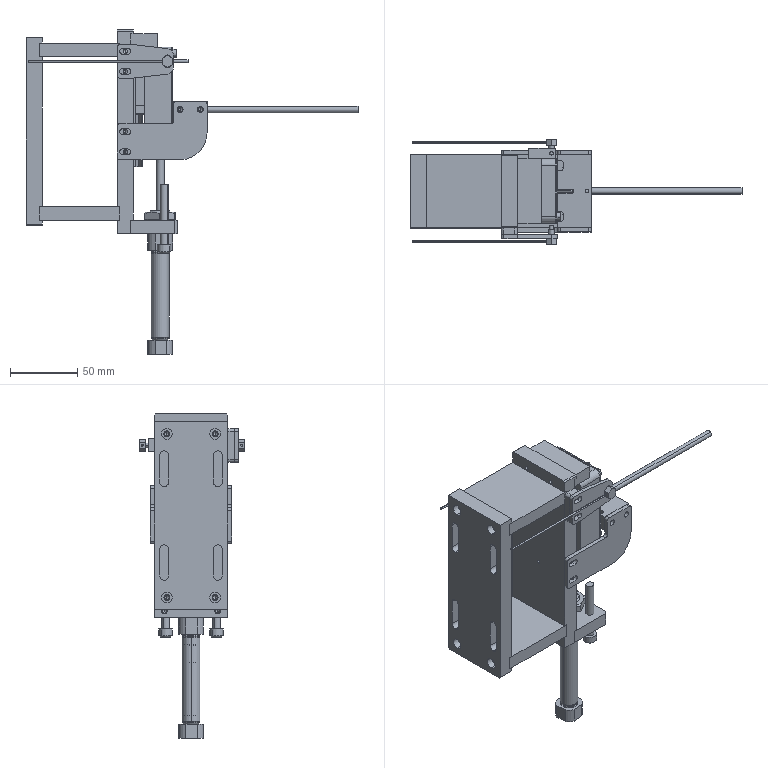Part | SolidWorks | features CompositeCurve 2 | 33 solids | 1048 faces | box 247.56 x 78.5 x 242 mm | volume 391168 mm3 | plane 517 | cylinder 375 | cone 126 | torus 14 | sphere 8 | spline 8 | commonest cylinder face diameters 3.3 x48 4 x38 2.5 x26 6 x24 4.4 x20 8 x20